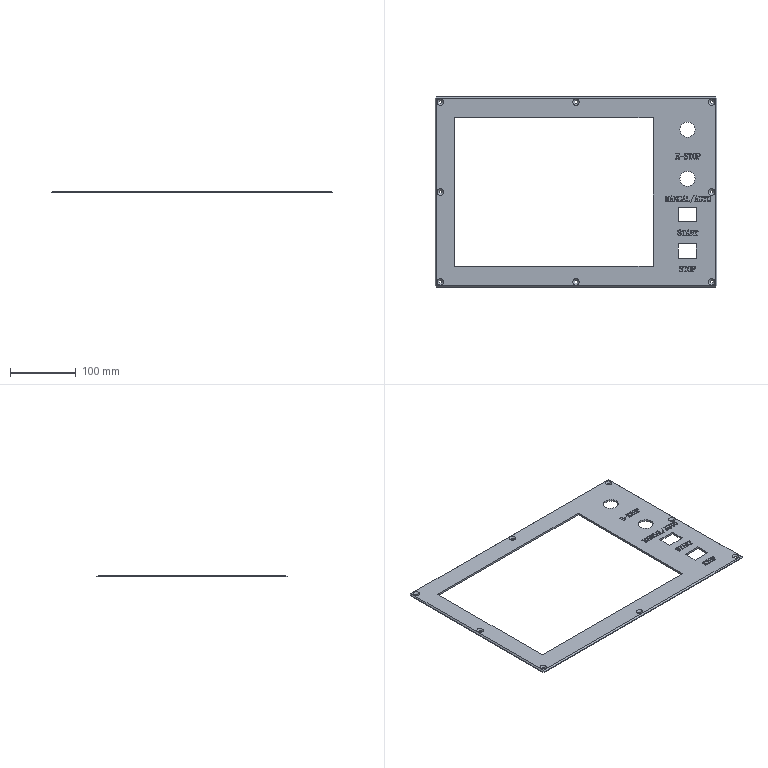Part | SolidWorks | features ICE 4, Chamfer 1, Extrusion 1, HoleWzd 1 | 1 solid | 599 faces | box 430 x 290 x 3 mm | volume 158728 mm3 | plane 386 | spline 177 | cylinder 20 | cone 16 | commonest cylinder face diameters 4.5 x16 23 x4